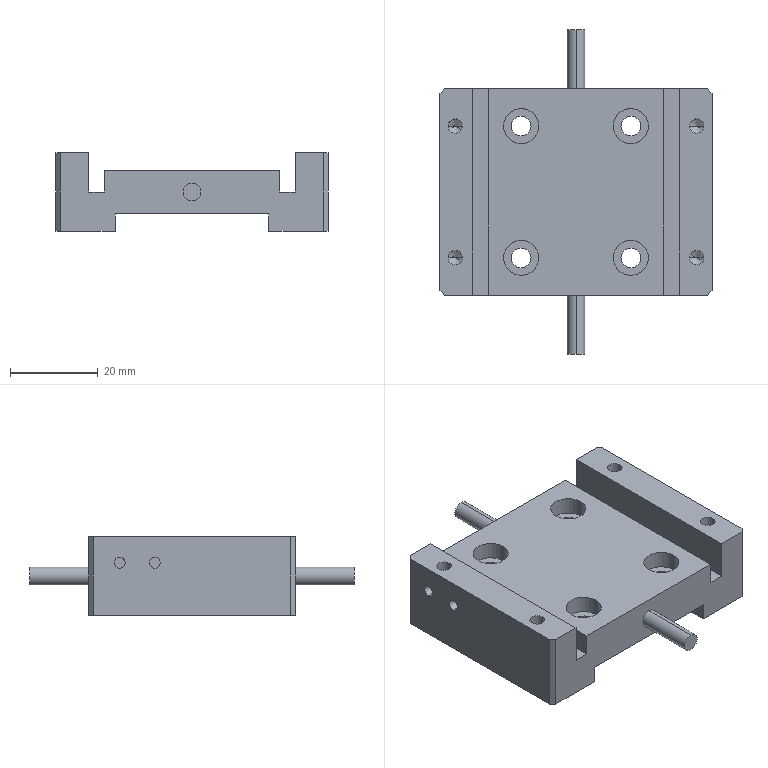Part | NX | features BREP 1 | 1 solid | 69 faces | box 62 x 74 x 18 mm | volume 34097 mm3 | cylinder 33 | plane 28 | cone 8 | commonest cylinder face diameters 3.3 x8 4.5 x8 8 x8 2.5 x5 4.076 x4